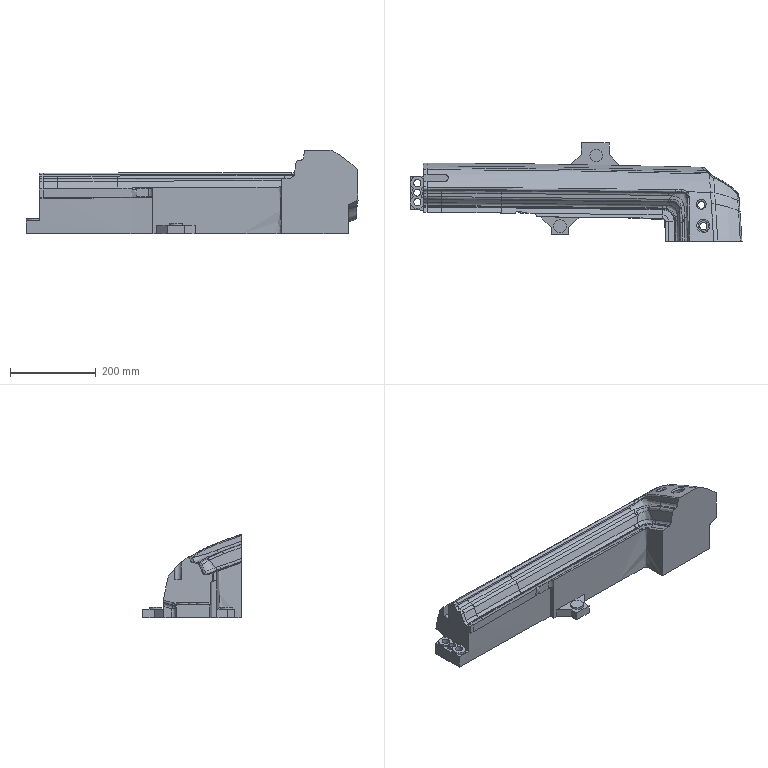Part | NX | features solid 2 | 1 solid | 197 faces | box 775.25 x 230.581 x 194.794 mm | volume 11045419 mm3 | spline 134 | plane 41 | cylinder 20 | sphere 2 | commonest cylinder face diameters 17 x4 32 x4 20 x3 25 x3 16 x2 30 x2